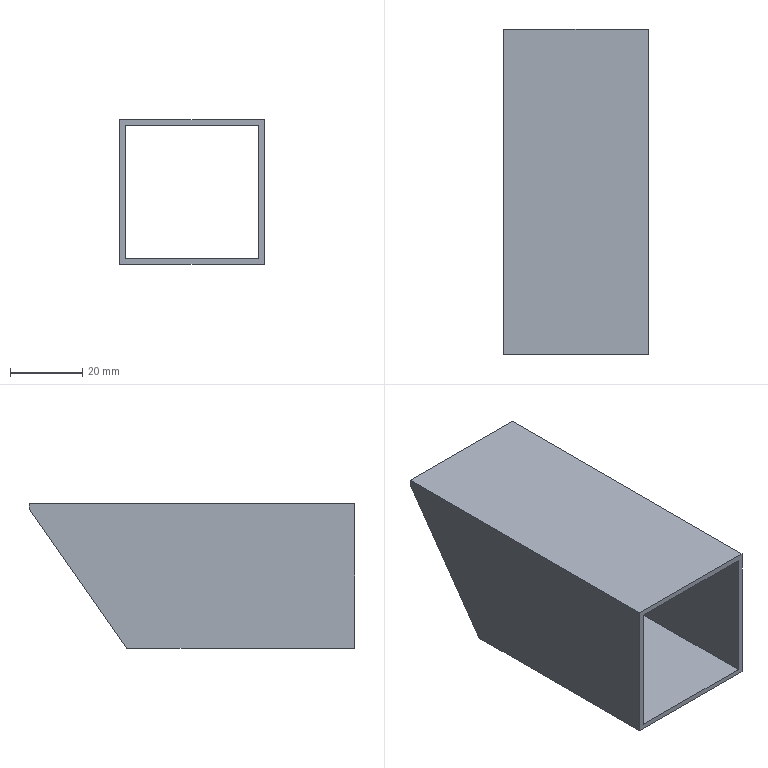Part | STEP file | 101 | 1 solid | 11 faces | box 40 x 90 x 40 mm | volume 17766 mm3 | plane 11
STEP:
#1=CARTESIAN_POINT('',(0.,0.,0.));
#2=DIRECTION('',(0.,0.,1.));
#3=DIRECTION('',(1.,0.,0.));
#4=AXIS2_PLACEMENT_3D('',#1,#2,#3);
#5=CARTESIAN_POINT('',(-20.,90.,18.5));
#6=VERTEX_POINT('',#5);
#7=CARTESIAN_POINT('',(-18.5,90.,18.5));
#8=VERTEX_POINT('',#7);
#9=CARTESIAN_POINT('',(0.,90.,18.5));
#10=DIRECTION('',(1.,0.,0.));
#11=VECTOR('',#10,1.);
#12=LINE('',#9,#11);
#13=CARTESIAN_POINT('',(0.,90.,0.));
#14=DIRECTION('',(0.,1.,0.));
#15=DIRECTION('',(0.,0.,1.));
#16=AXIS2_PLACEMENT_3D('',#13,#14,#15);
#17=PLANE('',#16);
#18=CARTESIAN_POINT('',(18.5,0.));
#19=DIRECTION('',(0.,1.));
#20=VECTOR('',#19,1.);
#21=LINE('',#18,#20);
#22=(GEOMETRIC_REPRESENTATION_CONTEXT(2)PARAMETRIC_REPRESENTATION_CONTEXT()REPRESENTATION_CONTEXT('',''));
#23=DEFINITIONAL_REPRESENTATION('',(#21),#22);
#24=PCURVE('',#17,#23);
#25=CARTESIAN_POINT('',(0.,51.699,-36.2));
#26=DIRECTION('',(0.,-0.8192,0.5736));
#27=DIRECTION('',(0.,-0.5736,-0.8192));
#28=AXIS2_PLACEMENT_3D('',#25,#26,#27);
#29=PLANE('',#28);
#30=CARTESIAN_POINT('',(-66.776,0.));
#31=DIRECTION('',(0.,1.));
#32=VECTOR('',#31,1.);
#33=LINE('',#30,#32);
#34=(GEOMETRIC_REPRESENTATION_CONTEXT(2)PARAMETRIC_REPRESENTATION_CONTEXT()REPRESENTATION_CONTEXT('',''));
#35=DEFINITIONAL_REPRESENTATION('',(#33),#34);
#36=PCURVE('',#29,#35);
#37=SURFACE_CURVE('',#12,(#24,#36),.PCURVE_S1.);
#38=EDGE_CURVE('',#6,#8,#37,.T.);
#39=ORIENTED_EDGE('',*,*,#38,.F.);
#40=CARTESIAN_POINT('',(-20.,90.,20.));
#41=VERTEX_POINT('',#40);
#42=CARTESIAN_POINT('',(-20.,90.,-20.));
#43=DIRECTION('',(0.,0.,1.));
#44=VECTOR('',#43,1.);
#45=LINE('',#42,#44);
#46=CARTESIAN_POINT('',(-20.,-20.));
#47=DIRECTION('',(1.,0.));
#48=VECTOR('',#47,1.);
#49=LINE('',#46,#48);
#50=(GEOMETRIC_REPRESENTATION_CONTEXT(2)PARAMETRIC_REPRESENTATION_CONTEXT()REPRESENTATION_CONTEXT('',''));
#51=DEFINITIONAL_REPRESENTATION('',(#49),#50);
#52=PCURVE('',#17,#51);
#53=CARTESIAN_POINT('',(-20.,90.,-20.));
#54=DIRECTION('',(1.,0.,0.));
#55=DIRECTION('',(0.,0.,-1.));
#56=AXIS2_PLACEMENT_3D('',#53,#54,#55);
#57=PLANE('',#56);
#58=CARTESIAN_POINT('',(0.,0.));
#59=DIRECTION('',(-1.,0.));
#60=VECTOR('',#59,1.);
#61=LINE('',#58,#60);
#62=(GEOMETRIC_REPRESENTATION_CONTEXT(2)PARAMETRIC_REPRESENTATION_CONTEXT()REPRESENTATION_CONTEXT('',''));
#63=DEFINITIONAL_REPRESENTATION('',(#61),#62);
#64=PCURVE('',#57,#63);
#65=SURFACE_CURVE('',#45,(#52,#64),.PCURVE_S1.);
#66=EDGE_CURVE('',#6,#41,#65,.T.);
#67=ORIENTED_EDGE('',*,*,#66,.T.);
#68=CARTESIAN_POINT('',(20.,90.,20.));
#69=VERTEX_POINT('',#68);
#70=CARTESIAN_POINT('',(-20.,90.,20.));
#71=DIRECTION('',(1.,0.,0.));
#72=VECTOR('',#71,1.);
#73=LINE('',#70,#72);
#74=CARTESIAN_POINT('',(20.,-20.));
#75=DIRECTION('',(0.,1.));
#76=VECTOR('',#75,1.);
#77=LINE('',#74,#76);
#78=(GEOMETRIC_REPRESENTATION_CONTEXT(2)PARAMETRIC_REPRESENTATION_CONTEXT()REPRESENTATION_CONTEXT('',''));
#79=DEFINITIONAL_REPRESENTATION('',(#77),#78);
#80=PCURVE('',#17,#79);
#81=CARTESIAN_POINT('',(-20.,90.,20.));
#82=DIRECTION('',(0.,0.,-1.));
#83=DIRECTION('',(-1.,0.,0.));
#84=AXIS2_PLACEMENT_3D('',#81,#82,#83);
#85=PLANE('',#84);
#86=CARTESIAN_POINT('',(0.,0.));
#87=DIRECTION('',(-1.,0.));
#88=VECTOR('',#87,1.);
#89=LINE('',#86,#88);
#90=(GEOMETRIC_REPRESENTATION_CONTEXT(2)PARAMETRIC_REPRESENTATION_CONTEXT()REPRESENTATION_CONTEXT('',''));
#91=DEFINITIONAL_REPRESENTATION('',(#89),#90);
#92=PCURVE('',#85,#91);
#93=SURFACE_CURVE('',#73,(#80,#92),.PCURVE_S1.);
#94=EDGE_CURVE('',#41,#69,#93,.T.);
#95=ORIENTED_EDGE('',*,*,#94,.T.);
#96=CARTESIAN_POINT('',(20.,90.,18.5));
#97=VERTEX_POINT('',#96);
#98=CARTESIAN_POINT('',(20.,90.,-20.));
#99=DIRECTION('',(0.,0.,-1.));
#100=VECTOR('',#99,1.);
#101=LINE('',#98,#100);
#102=CARTESIAN_POINT('',(-20.,20.));
#103=DIRECTION('',(-1.,0.));
#104=VECTOR('',#103,1.);
#105=LINE('',#102,#104);
#106=(GEOMETRIC_REPRESENTATION_CONTEXT(2)PARAMETRIC_REPRESENTATION_CONTEXT()REPRESENTATION_CONTEXT('',''));
#107=DEFINITIONAL_REPRESENTATION('',(#105),#106);
#108=PCURVE('',#17,#107);
#109=CARTESIAN_POINT('',(20.,90.,-20.));
#110=DIRECTION('',(-1.,0.,0.));
#111=DIRECTION('',(0.,0.,1.));
#112=AXIS2_PLACEMENT_3D('',#109,#110,#111);
#113=PLANE('',#112);
#114=CARTESIAN_POINT('',(0.,0.));
#115=DIRECTION('',(-1.,0.));
#116=VECTOR('',#115,1.);
#117=LINE('',#114,#116);
#118=(GEOMETRIC_REPRESENTATION_CONTEXT(2)PARAMETRIC_REPRESENTATION_CONTEXT()REPRESENTATION_CONTEXT('',''));
#119=DEFINITIONAL_REPRESENTATION('',(#117),#118);
#120=PCURVE('',#113,#119);
#121=SURFACE_CURVE('',#101,(#108,#120),.PCURVE_S1.);
#122=EDGE_CURVE('',#69,#97,#121,.T.);
#123=ORIENTED_EDGE('',*,*,#122,.T.);
#124=CARTESIAN_POINT('',(18.5,90.,18.5));
#125=VERTEX_POINT('',#124);
#126=CARTESIAN_POINT('',(0.,90.,18.5));
#127=DIRECTION('',(1.,0.,0.));
#128=VECTOR('',#127,1.);
#129=LINE('',#126,#128);
#130=CARTESIAN_POINT('',(18.5,0.));
#131=DIRECTION('',(0.,1.));
#132=VECTOR('',#131,1.);
#133=LINE('',#130,#132);
#134=(GEOMETRIC_REPRESENTATION_CONTEXT(2)PARAMETRIC_REPRESENTATION_CONTEXT()REPRESENTATION_CONTEXT('',''));
#135=DEFINITIONAL_REPRESENTATION('',(#133),#134);
#136=PCURVE('',#17,#135);
#137=CARTESIAN_POINT('',(-66.776,0.));
#138=DIRECTION('',(0.,1.));
#139=VECTOR('',#138,1.);
#140=LINE('',#137,#139);
#141=(GEOMETRIC_REPRESENTATION_CONTEXT(2)PARAMETRIC_REPRESENTATION_CONTEXT()REPRESENTATION_CONTEXT('',''));
#142=DEFINITIONAL_REPRESENTATION('',(#140),#141);
#143=PCURVE('',#29,#142);
#144=SURFACE_CURVE('',#129,(#136,#143),.PCURVE_S1.);
#145=EDGE_CURVE('',#125,#97,#144,.T.);
#146=ORIENTED_EDGE('',*,*,#145,.F.);
#147=CARTESIAN_POINT('',(-18.5,90.,18.5));
#148=DIRECTION('',(1.,0.,0.));
#149=VECTOR('',#148,1.);
#150=LINE('',#147,#149);
#151=CARTESIAN_POINT('',(18.5,-18.5));
#152=DIRECTION('',(0.,1.));
#153=VECTOR('',#152,1.);
#154=LINE('',#151,#153);
#155=(GEOMETRIC_REPRESENTATION_CONTEXT(2)PARAMETRIC_REPRESENTATION_CONTEXT()REPRESENTATION_CONTEXT('',''));
#156=DEFINITIONAL_REPRESENTATION('',(#154),#155);
#157=PCURVE('',#17,#156);
#158=CARTESIAN_POINT('',(-18.5,90.,18.5));
#159=DIRECTION('',(0.,0.,-1.));
#160=DIRECTION('',(-1.,0.,0.));
#161=AXIS2_PLACEMENT_3D('',#158,#159,#160);
#162=PLANE('',#161);
#163=CARTESIAN_POINT('',(0.,0.));
#164=DIRECTION('',(-1.,0.));
#165=VECTOR('',#164,1.);
#166=LINE('',#163,#165);
#167=(GEOMETRIC_REPRESENTATION_CONTEXT(2)PARAMETRIC_REPRESENTATION_CONTEXT()REPRESENTATION_CONTEXT('',''));
#168=DEFINITIONAL_REPRESENTATION('',(#166),#167);
#169=PCURVE('',#162,#168);
#170=SURFACE_CURVE('',#150,(#157,#169),.PCURVE_S1.);
#171=EDGE_CURVE('',#8,#125,#170,.T.);
#172=ORIENTED_EDGE('',*,*,#171,.F.);
#173=EDGE_LOOP('',(#39,#67,#95,#123,#146,#172));
#174=FACE_BOUND('',#173,.T.);
#175=ADVANCED_FACE('',(#174),#17,.T.);
#176=CARTESIAN_POINT('',(20.,0.,20.));
#177=VERTEX_POINT('',#176);
#178=CARTESIAN_POINT('',(20.,0.,-20.));
#179=VERTEX_POINT('',#178);
#180=CARTESIAN_POINT('',(20.,0.,-20.));
#181=DIRECTION('',(0.,0.,-1.));
#182=VECTOR('',#181,1.);
#183=LINE('',#180,#182);
#184=CARTESIAN_POINT('',(0.,0.,0.));
#185=DIRECTION('',(0.,1.,0.));
#186=DIRECTION('',(0.,0.,1.));
#187=AXIS2_PLACEMENT_3D('',#184,#185,#186);
#188=PLANE('',#187);
#189=CARTESIAN_POINT('',(-20.,20.));
#190=DIRECTION('',(-1.,0.));
#191=VECTOR('',#190,1.);
#192=LINE('',#189,#191);
#193=(GEOMETRIC_REPRESENTATION_CONTEXT(2)PARAMETRIC_REPRESENTATION_CONTEXT()REPRESENTATION_CONTEXT('',''));
#194=DEFINITIONAL_REPRESENTATION('',(#192),#193);
#195=PCURVE('',#188,#194);
#196=CARTESIAN_POINT('',(0.,-90.));
#197=DIRECTION('',(-1.,0.));
#198=VECTOR('',#197,1.);
#199=LINE('',#196,#198);
#200=(GEOMETRIC_REPRESENTATION_CONTEXT(2)PARAMETRIC_REPRESENTATION_CONTEXT()REPRESENTATION_CONTEXT('',''));
#201=DEFINITIONAL_REPRESENTATION('',(#199),#200);
#202=PCURVE('',#113,#201);
#203=SURFACE_CURVE('',#183,(#195,#202),.PCURVE_S1.);
#204=EDGE_CURVE('',#177,#179,#203,.T.);
#205=ORIENTED_EDGE('',*,*,#204,.F.);
#206=CARTESIAN_POINT('',(-20.,0.,20.));
#207=VERTEX_POINT('',#206);
#208=CARTESIAN_POINT('',(-20.,0.,20.));
#209=DIRECTION('',(1.,0.,0.));
#210=VECTOR('',#209,1.);
#211=LINE('',#208,#210);
#212=CARTESIAN_POINT('',(20.,-20.));
#213=DIRECTION('',(0.,1.));
#214=VECTOR('',#213,1.);
#215=LINE('',#212,#214);
#216=(GEOMETRIC_REPRESENTATION_CONTEXT(2)PARAMETRIC_REPRESENTATION_CONTEXT()REPRESENTATION_CONTEXT('',''));
#217=DEFINITIONAL_REPRESENTATION('',(#215),#216);
#218=PCURVE('',#188,#217);
#219=CARTESIAN_POINT('',(0.,-90.));
#220=DIRECTION('',(-1.,0.));
#221=VECTOR('',#220,1.);
#222=LINE('',#219,#221);
#223=(GEOMETRIC_REPRESENTATION_CONTEXT(2)PARAMETRIC_REPRESENTATION_CONTEXT()REPRESENTATION_CONTEXT('',''));
#224=DEFINITIONAL_REPRESENTATION('',(#222),#223);
#225=PCURVE('',#85,#224);
#226=SURFACE_CURVE('',#211,(#218,#225),.PCURVE_S1.);
#227=EDGE_CURVE('',#207,#177,#226,.T.);
#228=ORIENTED_EDGE('',*,*,#227,.F.);
#229=CARTESIAN_POINT('',(-20.,0.,-20.));
#230=VERTEX_POINT('',#229);
#231=CARTESIAN_POINT('',(-20.,0.,-20.));
#232=DIRECTION('',(0.,0.,1.));
#233=VECTOR('',#232,1.);
#234=LINE('',#231,#233);
#235=CARTESIAN_POINT('',(-20.,-20.));
#236=DIRECTION('',(1.,0.));
#237=VECTOR('',#236,1.);
#238=LINE('',#235,#237);
#239=(GEOMETRIC_REPRESENTATION_CONTEXT(2)PARAMETRIC_REPRESENTATION_CONTEXT()REPRESENTATION_CONTEXT('',''));
#240=DEFINITIONAL_REPRESENTATION('',(#238),#239);
#241=PCURVE('',#188,#240);
#242=CARTESIAN_POINT('',(0.,-90.));
#243=DIRECTION('',(-1.,0.));
#244=VECTOR('',#243,1.);
#245=LINE('',#242,#244);
#246=(GEOMETRIC_REPRESENTATION_CONTEXT(2)PARAMETRIC_REPRESENTATION_CONTEXT()REPRESENTATION_CONTEXT('',''));
#247=DEFINITIONAL_REPRESENTATION('',(#245),#246);
#248=PCURVE('',#57,#247);
#249=SURFACE_CURVE('',#234,(#241,#248),.PCURVE_S1.);
#250=EDGE_CURVE('',#230,#207,#249,.T.);
#251=ORIENTED_EDGE('',*,*,#250,.F.);
#252=CARTESIAN_POINT('',(-20.,0.,-20.));
#253=DIRECTION('',(-1.,0.,0.));
#254=VECTOR('',#253,1.);
#255=LINE('',#252,#254);
#256=CARTESIAN_POINT('',(-20.,-20.));
#257=DIRECTION('',(0.,-1.));
#258=VECTOR('',#257,1.);
#259=LINE('',#256,#258);
#260=(GEOMETRIC_REPRESENTATION_CONTEXT(2)PARAMETRIC_REPRESENTATION_CONTEXT()REPRESENTATION_CONTEXT('',''));
#261=DEFINITIONAL_REPRESENTATION('',(#259),#260);
#262=PCURVE('',#188,#261);
#263=CARTESIAN_POINT('',(-20.,90.,-20.));
#264=DIRECTION('',(0.,0.,1.));
#265=DIRECTION('',(1.,0.,0.));
#266=AXIS2_PLACEMENT_3D('',#263,#264,#265);
#267=PLANE('',#266);
#268=CARTESIAN_POINT('',(0.,-90.));
#269=DIRECTION('',(-1.,0.));
#270=VECTOR('',#269,1.);
#271=LINE('',#268,#270);
#272=(GEOMETRIC_REPRESENTATION_CONTEXT(2)PARAMETRIC_REPRESENTATION_CONTEXT()REPRESENTATION_CONTEXT('',''));
#273=DEFINITIONAL_REPRESENTATION('',(#271),#272);
#274=PCURVE('',#267,#273);
#275=SURFACE_CURVE('',#255,(#262,#274),.PCURVE_S1.);
#276=EDGE_CURVE('',#179,#230,#275,.T.);
#277=ORIENTED_EDGE('',*,*,#276,.F.);
#278=EDGE_LOOP('',(#205,#228,#251,#277));
#279=FACE_BOUND('',#278,.T.);
#280=CARTESIAN_POINT('',(18.5,0.,18.5));
#281=VERTEX_POINT('',#280);
#282=CARTESIAN_POINT('',(18.5,0.,-18.5));
#283=VERTEX_POINT('',#282);
#284=CARTESIAN_POINT('',(18.5,0.,-18.5));
#285=DIRECTION('',(0.,0.,-1.));
#286=VECTOR('',#285,1.);
#287=LINE('',#284,#286);
#288=CARTESIAN_POINT('',(-18.5,18.5));
#289=DIRECTION('',(-1.,0.));
#290=VECTOR('',#289,1.);
#291=LINE('',#288,#290);
#292=(GEOMETRIC_REPRESENTATION_CONTEXT(2)PARAMETRIC_REPRESENTATION_CONTEXT()REPRESENTATION_CONTEXT('',''));
#293=DEFINITIONAL_REPRESENTATION('',(#291),#292);
#294=PCURVE('',#188,#293);
#295=CARTESIAN_POINT('',(18.5,90.,-18.5));
#296=DIRECTION('',(-1.,0.,0.));
#297=DIRECTION('',(0.,0.,1.));
#298=AXIS2_PLACEMENT_3D('',#295,#296,#297);
#299=PLANE('',#298);
#300=CARTESIAN_POINT('',(0.,-90.));
#301=DIRECTION('',(-1.,0.));
#302=VECTOR('',#301,1.);
#303=LINE('',#300,#302);
#304=(GEOMETRIC_REPRESENTATION_CONTEXT(2)PARAMETRIC_REPRESENTATION_CONTEXT()REPRESENTATION_CONTEXT('',''));
#305=DEFINITIONAL_REPRESENTATION('',(#303),#304);
#306=PCURVE('',#299,#305);
#307=SURFACE_CURVE('',#287,(#294,#306),.PCURVE_S1.);
#308=EDGE_CURVE('',#281,#283,#307,.T.);
#309=ORIENTED_EDGE('',*,*,#308,.T.);
#310=CARTESIAN_POINT('',(-18.5,0.,-18.5));
#311=VERTEX_POINT('',#310);
#312=CARTESIAN_POINT('',(-18.5,0.,-18.5));
#313=DIRECTION('',(-1.,0.,0.));
#314=VECTOR('',#313,1.);
#315=LINE('',#312,#314);
#316=CARTESIAN_POINT('',(-18.5,-18.5));
#317=DIRECTION('',(0.,-1.));
#318=VECTOR('',#317,1.);
#319=LINE('',#316,#318);
#320=(GEOMETRIC_REPRESENTATION_CONTEXT(2)PARAMETRIC_REPRESENTATION_CONTEXT()REPRESENTATION_CONTEXT('',''));
#321=DEFINITIONAL_REPRESENTATION('',(#319),#320);
#322=PCURVE('',#188,#321);
#323=CARTESIAN_POINT('',(-18.5,90.,-18.5));
#324=DIRECTION('',(0.,0.,1.));
#325=DIRECTION('',(1.,0.,0.));
#326=AXIS2_PLACEMENT_3D('',#323,#324,#325);
#327=PLANE('',#326);
#328=CARTESIAN_POINT('',(0.,-90.));
#329=DIRECTION('',(-1.,0.));
#330=VECTOR('',#329,1.);
#331=LINE('',#328,#330);
#332=(GEOMETRIC_REPRESENTATION_CONTEXT(2)PARAMETRIC_REPRESENTATION_CONTEXT()REPRESENTATION_CONTEXT('',''));
#333=DEFINITIONAL_REPRESENTATION('',(#331),#332);
#334=PCURVE('',#327,#333);
#335=SURFACE_CURVE('',#315,(#322,#334),.PCURVE_S1.);
#336=EDGE_CURVE('',#283,#311,#335,.T.);
#337=ORIENTED_EDGE('',*,*,#336,.T.);
#338=CARTESIAN_POINT('',(-18.5,0.,18.5));
#339=VERTEX_POINT('',#338);
#340=CARTESIAN_POINT('',(-18.5,0.,-18.5));
#341=DIRECTION('',(0.,0.,1.));
#342=VECTOR('',#341,1.);
#343=LINE('',#340,#342);
#344=CARTESIAN_POINT('',(-18.5,-18.5));
#345=DIRECTION('',(1.,0.));
#346=VECTOR('',#345,1.);
#347=LINE('',#344,#346);
#348=(GEOMETRIC_REPRESENTATION_CONTEXT(2)PARAMETRIC_REPRESENTATION_CONTEXT()REPRESENTATION_CONTEXT('',''));
#349=DEFINITIONAL_REPRESENTATION('',(#347),#348);
#350=PCURVE('',#188,#349);
#351=CARTESIAN_POINT('',(-18.5,90.,-18.5));
#352=DIRECTION('',(1.,0.,0.));
#353=DIRECTION('',(0.,0.,-1.));
#354=AXIS2_PLACEMENT_3D('',#351,#352,#353);
#355=PLANE('',#354);
#356=CARTESIAN_POINT('',(0.,-90.));
#357=DIRECTION('',(-1.,0.));
#358=VECTOR('',#357,1.);
#359=LINE('',#356,#358);
#360=(GEOMETRIC_REPRESENTATION_CONTEXT(2)PARAMETRIC_REPRESENTATION_CONTEXT()REPRESENTATION_CONTEXT('',''));
#361=DEFINITIONAL_REPRESENTATION('',(#359),#360);
#362=PCURVE('',#355,#361);
#363=SURFACE_CURVE('',#343,(#350,#362),.PCURVE_S1.);
#364=EDGE_CURVE('',#311,#339,#363,.T.);
#365=ORIENTED_EDGE('',*,*,#364,.T.);
#366=CARTESIAN_POINT('',(-18.5,0.,18.5));
#367=DIRECTION('',(1.,0.,0.));
#368=VECTOR('',#367,1.);
#369=LINE('',#366,#368);
#370=CARTESIAN_POINT('',(18.5,-18.5));
#371=DIRECTION('',(0.,1.));
#372=VECTOR('',#371,1.);
#373=LINE('',#370,#372);
#374=(GEOMETRIC_REPRESENTATION_CONTEXT(2)PARAMETRIC_REPRESENTATION_CONTEXT()REPRESENTATION_CONTEXT('',''));
#375=DEFINITIONAL_REPRESENTATION('',(#373),#374);
#376=PCURVE('',#188,#375);
#377=CARTESIAN_POINT('',(0.,-90.));
#378=DIRECTION('',(-1.,0.));
#379=VECTOR('',#378,1.);
#380=LINE('',#377,#379);
#381=(GEOMETRIC_REPRESENTATION_CONTEXT(2)PARAMETRIC_REPRESENTATION_CONTEXT()REPRESENTATION_CONTEXT('',''));
#382=DEFINITIONAL_REPRESENTATION('',(#380),#381);
#383=PCURVE('',#162,#382);
#384=SURFACE_CURVE('',#369,(#376,#383),.PCURVE_S1.);
#385=EDGE_CURVE('',#339,#281,#384,.T.);
#386=ORIENTED_EDGE('',*,*,#385,.T.);
#387=EDGE_LOOP('',(#309,#337,#365,#386));
#388=FACE_BOUND('',#387,.T.);
#389=ADVANCED_FACE('',(#279,#388),#188,.F.);
#390=CARTESIAN_POINT('',(20.,63.042,-20.));
#391=VERTEX_POINT('',#390);
#392=CARTESIAN_POINT('',(20.,90.,-20.));
#393=DIRECTION('',(0.,-1.,0.));
#394=VECTOR('',#393,1.);
#395=LINE('',#392,#394);
#396=CARTESIAN_POINT('',(0.,0.));
#397=DIRECTION('',(0.,-1.));
#398=VECTOR('',#397,1.);
#399=LINE('',#396,#398);
#400=(GEOMETRIC_REPRESENTATION_CONTEXT(2)PARAMETRIC_REPRESENTATION_CONTEXT()REPRESENTATION_CONTEXT('',''));
#401=DEFINITIONAL_REPRESENTATION('',(#399),#400);
#402=PCURVE('',#113,#401);
#403=CARTESIAN_POINT('',(40.,0.));
#404=DIRECTION('',(0.,-1.));
#405=VECTOR('',#404,1.);
#406=LINE('',#403,#405);
#407=(GEOMETRIC_REPRESENTATION_CONTEXT(2)PARAMETRIC_REPRESENTATION_CONTEXT()REPRESENTATION_CONTEXT('',''));
#408=DEFINITIONAL_REPRESENTATION('',(#406),#407);
#409=PCURVE('',#267,#408);
#410=SURFACE_CURVE('',#395,(#402,#409),.PCURVE_S1.);
#411=EDGE_CURVE('',#391,#179,#410,.T.);
#412=ORIENTED_EDGE('',*,*,#411,.F.);
#413=CARTESIAN_POINT('',(20.,71.911,-7.334));
#414=DIRECTION('',(0.,0.5736,0.8192));
#415=VECTOR('',#414,1.);
#416=LINE('',#413,#415);
#417=CARTESIAN_POINT('',(12.666,-18.089));
#418=DIRECTION('',(0.8192,0.5736));
#419=VECTOR('',#418,1.);
#420=LINE('',#417,#419);
#421=(GEOMETRIC_REPRESENTATION_CONTEXT(2)PARAMETRIC_REPRESENTATION_CONTEXT()REPRESENTATION_CONTEXT('',''));
#422=DEFINITIONAL_REPRESENTATION('',(#420),#421);
#423=PCURVE('',#113,#422);
#424=CARTESIAN_POINT('',(-35.239,20.));
#425=DIRECTION('',(-1.,0.));
#426=VECTOR('',#425,1.);
#427=LINE('',#424,#426);
#428=(GEOMETRIC_REPRESENTATION_CONTEXT(2)PARAMETRIC_REPRESENTATION_CONTEXT()REPRESENTATION_CONTEXT('',''));
#429=DEFINITIONAL_REPRESENTATION('',(#427),#428);
#430=PCURVE('',#29,#429);
#431=SURFACE_CURVE('',#416,(#423,#430),.PCURVE_S1.);
#432=EDGE_CURVE('',#391,#97,#431,.T.);
#433=ORIENTED_EDGE('',*,*,#432,.T.);
#434=ORIENTED_EDGE('',*,*,#122,.F.);
#435=CARTESIAN_POINT('',(20.,90.,20.));
#436=DIRECTION('',(0.,-1.,0.));
#437=VECTOR('',#436,1.);
#438=LINE('',#435,#437);
#439=CARTESIAN_POINT('',(40.,0.));
#440=DIRECTION('',(0.,-1.));
#441=VECTOR('',#440,1.);
#442=LINE('',#439,#441);
#443=(GEOMETRIC_REPRESENTATION_CONTEXT(2)PARAMETRIC_REPRESENTATION_CONTEXT()REPRESENTATION_CONTEXT('',''));
#444=DEFINITIONAL_REPRESENTATION('',(#442),#443);
#445=PCURVE('',#113,#444);
#446=CARTESIAN_POINT('',(-40.,0.));
#447=DIRECTION('',(0.,-1.));
#448=VECTOR('',#447,1.);
#449=LINE('',#446,#448);
#450=(GEOMETRIC_REPRESENTATION_CONTEXT(2)PARAMETRIC_REPRESENTATION_CONTEXT()REPRESENTATION_CONTEXT('',''));
#451=DEFINITIONAL_REPRESENTATION('',(#449),#450);
#452=PCURVE('',#85,#451);
#453=SURFACE_CURVE('',#438,(#445,#452),.PCURVE_S1.);
#454=EDGE_CURVE('',#69,#177,#453,.T.);
#455=ORIENTED_EDGE('',*,*,#454,.T.);
#456=ORIENTED_EDGE('',*,*,#204,.T.);
#457=EDGE_LOOP('',(#412,#433,#434,#455,#456));
#458=FACE_BOUND('',#457,.T.);
#459=ADVANCED_FACE('',(#458),#113,.F.);
#460=CARTESIAN_POINT('',(-20.,63.042,-20.));
#461=VERTEX_POINT('',#460);
#462=CARTESIAN_POINT('',(-20.,90.,-20.));
#463=DIRECTION('',(0.,-1.,0.));
#464=VECTOR('',#463,1.);
#465=LINE('',#462,#464);
#466=CARTESIAN_POINT('',(0.,0.));
#467=DIRECTION('',(0.,-1.));
#468=VECTOR('',#467,1.);
#469=LINE('',#466,#468);
#470=(GEOMETRIC_REPRESENTATION_CONTEXT(2)PARAMETRIC_REPRESENTATION_CONTEXT()REPRESENTATION_CONTEXT('',''));
#471=DEFINITIONAL_REPRESENTATION('',(#469),#470);
#472=PCURVE('',#267,#471);
#473=CARTESIAN_POINT('',(0.,0.));
#474=DIRECTION('',(0.,-1.));
#475=VECTOR('',#474,1.);
#476=LINE('',#473,#475);
#477=(GEOMETRIC_REPRESENTATION_CONTEXT(2)PARAMETRIC_REPRESENTATION_CONTEXT()REPRESENTATION_CONTEXT('',''));
#478=DEFINITIONAL_REPRESENTATION('',(#476),#477);
#479=PCURVE('',#57,#478);
#480=SURFACE_CURVE('',#465,(#472,#479),.PCURVE_S1.);
#481=EDGE_CURVE('',#461,#230,#480,.T.);
#482=ORIENTED_EDGE('',*,*,#481,.F.);
#483=CARTESIAN_POINT('',(-20.,63.042,-20.));
#484=DIRECTION('',(1.,0.,0.));
#485=VECTOR('',#484,1.);
#486=LINE('',#483,#485);
#487=CARTESIAN_POINT('',(0.,-26.958));
#488=DIRECTION('',(1.,0.));
#489=VECTOR('',#488,1.);
#490=LINE('',#487,#489);
#491=(GEOMETRIC_REPRESENTATION_CONTEXT(2)PARAMETRIC_REPRESENTATION_CONTEXT()REPRESENTATION_CONTEXT('',''));
#492=DEFINITIONAL_REPRESENTATION('',(#490),#491);
#493=PCURVE('',#267,#492);
#494=CARTESIAN_POINT('',(-19.776,-20.));
#495=DIRECTION('',(0.,1.));
#496=VECTOR('',#495,1.);
#497=LINE('',#494,#496);
#498=(GEOMETRIC_REPRESENTATION_CONTEXT(2)PARAMETRIC_REPRESENTATION_CONTEXT()REPRESENTATION_CONTEXT('',''));
#499=DEFINITIONAL_REPRESENTATION('',(#497),#498);
#500=PCURVE('',#29,#499);
#501=SURFACE_CURVE('',#486,(#493,#500),.PCURVE_S1.);
#502=EDGE_CURVE('',#461,#391,#501,.T.);
#503=ORIENTED_EDGE('',*,*,#502,.T.);
#504=ORIENTED_EDGE('',*,*,#411,.T.);
#505=ORIENTED_EDGE('',*,*,#276,.T.);
#506=EDGE_LOOP('',(#482,#503,#504,#505));
#507=FACE_BOUND('',#506,.T.);
#508=ADVANCED_FACE('',(#507),#267,.F.);
#509=ORIENTED_EDGE('',*,*,#66,.F.);
#510=CARTESIAN_POINT('',(-20.,71.911,-7.334));
#511=DIRECTION('',(0.,-0.5736,-0.8192));
#512=VECTOR('',#511,1.);
#513=LINE('',#510,#512);
#514=CARTESIAN_POINT('',(-12.666,-18.089));
#515=DIRECTION('',(0.8192,-0.5736));
#516=VECTOR('',#515,1.);
#517=LINE('',#514,#516);
#518=(GEOMETRIC_REPRESENTATION_CONTEXT(2)PARAMETRIC_REPRESENTATION_CONTEXT()REPRESENTATION_CONTEXT('',''));
#519=DEFINITIONAL_REPRESENTATION('',(#517),#518);
#520=PCURVE('',#57,#519);
#521=CARTESIAN_POINT('',(-35.239,-20.));
#522=DIRECTION('',(1.,0.));
#523=VECTOR('',#522,1.);
#524=LINE('',#521,#523);
#525=(GEOMETRIC_REPRESENTATION_CONTEXT(2)PARAMETRIC_REPRESENTATION_CONTEXT()REPRESENTATION_CONTEXT('',''));
#526=DEFINITIONAL_REPRESENTATION('',(#524),#525);
#527=PCURVE('',#29,#526);
#528=SURFACE_CURVE('',#513,(#520,#527),.PCURVE_S1.);
#529=EDGE_CURVE('',#6,#461,#528,.T.);
#530=ORIENTED_EDGE('',*,*,#529,.T.);
#531=ORIENTED_EDGE('',*,*,#481,.T.);
#532=ORIENTED_EDGE('',*,*,#250,.T.);
#533=CARTESIAN_POINT('',(-20.,90.,20.));
#534=DIRECTION('',(0.,-1.,0.));
#535=VECTOR('',#534,1.);
#536=LINE('',#533,#535);
#537=CARTESIAN_POINT('',(-40.,0.));
#538=DIRECTION('',(0.,-1.));
#539=VECTOR('',#538,1.);
#540=LINE('',#537,#539);
#541=(GEOMETRIC_REPRESENTATION_CONTEXT(2)PARAMETRIC_REPRESENTATION_CONTEXT()REPRESENTATION_CONTEXT('',''));
#542=DEFINITIONAL_REPRESENTATION('',(#540),#541);
#543=PCURVE('',#57,#542);
#544=CARTESIAN_POINT('',(0.,0.));
#545=DIRECTION('',(0.,-1.));
#546=VECTOR('',#545,1.);
#547=LINE('',#544,#546);
#548=(GEOMETRIC_REPRESENTATION_CONTEXT(2)PARAMETRIC_REPRESENTATION_CONTEXT()REPRESENTATION_CONTEXT('',''));
#549=DEFINITIONAL_REPRESENTATION('',(#547),#548);
#550=PCURVE('',#85,#549);
#551=SURFACE_CURVE('',#536,(#543,#550),.PCURVE_S1.);
#552=EDGE_CURVE('',#41,#207,#551,.T.);
#553=ORIENTED_EDGE('',*,*,#552,.F.);
#554=EDGE_LOOP('',(#509,#530,#531,#532,#553));
#555=FACE_BOUND('',#554,.T.);
#556=ADVANCED_FACE('',(#555),#57,.F.);
#557=ORIENTED_EDGE('',*,*,#227,.T.);
#558=ORIENTED_EDGE('',*,*,#454,.F.);
#559=ORIENTED_EDGE('',*,*,#94,.F.);
#560=ORIENTED_EDGE('',*,*,#552,.T.);
#561=EDGE_LOOP('',(#557,#558,#559,#560));
#562=FACE_BOUND('',#561,.T.);
#563=ADVANCED_FACE('',(#562),#85,.F.);
#564=CARTESIAN_POINT('',(18.5,64.092,-18.5));
#565=VERTEX_POINT('',#564);
#566=CARTESIAN_POINT('',(18.5,72.616,-6.327));
#567=DIRECTION('',(0.,0.5736,0.8192));
#568=VECTOR('',#567,1.);
#569=LINE('',#566,#568);
#570=CARTESIAN_POINT('',(12.173,-17.384));
#571=DIRECTION('',(0.8192,0.5736));
#572=VECTOR('',#571,1.);
#573=LINE('',#570,#572);
#574=(GEOMETRIC_REPRESENTATION_CONTEXT(2)PARAMETRIC_REPRESENTATION_CONTEXT()REPRESENTATION_CONTEXT('',''));
#575=DEFINITIONAL_REPRESENTATION('',(#573),#574);
#576=PCURVE('',#299,#575);
#577=CARTESIAN_POINT('',(-36.468,18.5));
#578=DIRECTION('',(-1.,0.));
#579=VECTOR('',#578,1.);
#580=LINE('',#577,#579);
#581=(GEOMETRIC_REPRESENTATION_CONTEXT(2)PARAMETRIC_REPRESENTATION_CONTEXT()REPRESENTATION_CONTEXT('',''));
#582=DEFINITIONAL_REPRESENTATION('',(#580),#581);
#583=PCURVE('',#29,#582);
#584=SURFACE_CURVE('',#569,(#576,#583),.PCURVE_S1.);
#585=EDGE_CURVE('',#565,#125,#584,.T.);
#586=ORIENTED_EDGE('',*,*,#585,.F.);
#587=CARTESIAN_POINT('',(18.5,90.,-18.5));
#588=DIRECTION('',(0.,-1.,0.));
#589=VECTOR('',#588,1.);
#590=LINE('',#587,#589);
#591=CARTESIAN_POINT('',(0.,0.));
#592=DIRECTION('',(0.,-1.));
#593=VECTOR('',#592,1.);
#594=LINE('',#591,#593);
#595=(GEOMETRIC_REPRESENTATION_CONTEXT(2)PARAMETRIC_REPRESENTATION_CONTEXT()REPRESENTATION_CONTEXT('',''));
#596=DEFINITIONAL_REPRESENTATION('',(#594),#595);
#597=PCURVE('',#299,#596);
#598=CARTESIAN_POINT('',(37.,0.));
#599=DIRECTION('',(0.,-1.));
#600=VECTOR('',#599,1.);
#601=LINE('',#598,#600);
#602=(GEOMETRIC_REPRESENTATION_CONTEXT(2)PARAMETRIC_REPRESENTATION_CONTEXT()REPRESENTATION_CONTEXT('',''));
#603=DEFINITIONAL_REPRESENTATION('',(#601),#602);
#604=PCURVE('',#327,#603);
#605=SURFACE_CURVE('',#590,(#597,#604),.PCURVE_S1.);
#606=EDGE_CURVE('',#565,#283,#605,.T.);
#607=ORIENTED_EDGE('',*,*,#606,.T.);
#608=ORIENTED_EDGE('',*,*,#308,.F.);
#609=CARTESIAN_POINT('',(18.5,90.,18.5));
#610=DIRECTION('',(0.,-1.,0.));
#611=VECTOR('',#610,1.);
#612=LINE('',#609,#611);
#613=CARTESIAN_POINT('',(37.,0.));
#614=DIRECTION('',(0.,-1.));
#615=VECTOR('',#614,1.);
#616=LINE('',#613,#615);
#617=(GEOMETRIC_REPRESENTATION_CONTEXT(2)PARAMETRIC_REPRESENTATION_CONTEXT()REPRESENTATION_CONTEXT('',''));
#618=DEFINITIONAL_REPRESENTATION('',(#616),#617);
#619=PCURVE('',#299,#618);
#620=CARTESIAN_POINT('',(-37.,0.));
#621=DIRECTION('',(0.,-1.));
#622=VECTOR('',#621,1.);
#623=LINE('',#620,#622);
#624=(GEOMETRIC_REPRESENTATION_CONTEXT(2)PARAMETRIC_REPRESENTATION_CONTEXT()REPRESENTATION_CONTEXT('',''));
#625=DEFINITIONAL_REPRESENTATION('',(#623),#624);
#626=PCURVE('',#162,#625);
#627=SURFACE_CURVE('',#612,(#619,#626),.PCURVE_S1.);
#628=EDGE_CURVE('',#125,#281,#627,.T.);
#629=ORIENTED_EDGE('',*,*,#628,.F.);
#630=EDGE_LOOP('',(#586,#607,#608,#629));
#631=FACE_BOUND('',#630,.T.);
#632=ADVANCED_FACE('',(#631),#299,.T.);
#633=CARTESIAN_POINT('',(-18.5,64.092,-18.5));
#634=VERTEX_POINT('',#633);
#635=CARTESIAN_POINT('',(-18.5,64.092,-18.5));
#636=DIRECTION('',(1.,0.,0.));
#637=VECTOR('',#636,1.);
#638=LINE('',#635,#637);
#639=CARTESIAN_POINT('',(0.,-25.908));
#640=DIRECTION('',(1.,0.));
#641=VECTOR('',#640,1.);
#642=LINE('',#639,#641);
#643=(GEOMETRIC_REPRESENTATION_CONTEXT(2)PARAMETRIC_REPRESENTATION_CONTEXT()REPRESENTATION_CONTEXT('',''));
#644=DEFINITIONAL_REPRESENTATION('',(#642),#643);
#645=PCURVE('',#327,#644);
#646=CARTESIAN_POINT('',(-21.608,-18.5));
#647=DIRECTION('',(0.,1.));
#648=VECTOR('',#647,1.);
#649=LINE('',#646,#648);
#650=(GEOMETRIC_REPRESENTATION_CONTEXT(2)PARAMETRIC_REPRESENTATION_CONTEXT()REPRESENTATION_CONTEXT('',''));
#651=DEFINITIONAL_REPRESENTATION('',(#649),#650);
#652=PCURVE('',#29,#651);
#653=SURFACE_CURVE('',#638,(#645,#652),.PCURVE_S1.);
#654=EDGE_CURVE('',#634,#565,#653,.T.);
#655=ORIENTED_EDGE('',*,*,#654,.F.);
#656=CARTESIAN_POINT('',(-18.5,90.,-18.5));
#657=DIRECTION('',(0.,-1.,0.));
#658=VECTOR('',#657,1.);
#659=LINE('',#656,#658);
#660=CARTESIAN_POINT('',(0.,0.));
#661=DIRECTION('',(0.,-1.));
#662=VECTOR('',#661,1.);
#663=LINE('',#660,#662);
#664=(GEOMETRIC_REPRESENTATION_CONTEXT(2)PARAMETRIC_REPRESENTATION_CONTEXT()REPRESENTATION_CONTEXT('',''));
#665=DEFINITIONAL_REPRESENTATION('',(#663),#664);
#666=PCURVE('',#327,#665);
#667=CARTESIAN_POINT('',(0.,0.));
#668=DIRECTION('',(0.,-1.));
#669=VECTOR('',#668,1.);
#670=LINE('',#667,#669);
#671=(GEOMETRIC_REPRESENTATION_CONTEXT(2)PARAMETRIC_REPRESENTATION_CONTEXT()REPRESENTATION_CONTEXT('',''));
#672=DEFINITIONAL_REPRESENTATION('',(#670),#671);
#673=PCURVE('',#355,#672);
#674=SURFACE_CURVE('',#659,(#666,#673),.PCURVE_S1.);
#675=EDGE_CURVE('',#634,#311,#674,.T.);
#676=ORIENTED_EDGE('',*,*,#675,.T.);
#677=ORIENTED_EDGE('',*,*,#336,.F.);
#678=ORIENTED_EDGE('',*,*,#606,.F.);
#679=EDGE_LOOP('',(#655,#676,#677,#678));
#680=FACE_BOUND('',#679,.T.);
#681=ADVANCED_FACE('',(#680),#327,.T.);
#682=CARTESIAN_POINT('',(-18.5,72.616,-6.327));
#683=DIRECTION('',(0.,-0.5736,-0.8192));
#684=VECTOR('',#683,1.);
#685=LINE('',#682,#684);
#686=CARTESIAN_POINT('',(-12.173,-17.384));
#687=DIRECTION('',(0.8192,-0.5736));
#688=VECTOR('',#687,1.);
#689=LINE('',#686,#688);
#690=(GEOMETRIC_REPRESENTATION_CONTEXT(2)PARAMETRIC_REPRESENTATION_CONTEXT()REPRESENTATION_CONTEXT('',''));
#691=DEFINITIONAL_REPRESENTATION('',(#689),#690);
#692=PCURVE('',#355,#691);
#693=CARTESIAN_POINT('',(-36.468,-18.5));
#694=DIRECTION('',(1.,0.));
#695=VECTOR('',#694,1.);
#696=LINE('',#693,#695);
#697=(GEOMETRIC_REPRESENTATION_CONTEXT(2)PARAMETRIC_REPRESENTATION_CONTEXT()REPRESENTATION_CONTEXT('',''));
#698=DEFINITIONAL_REPRESENTATION('',(#696),#697);
#699=PCURVE('',#29,#698);
#700=SURFACE_CURVE('',#685,(#692,#699),.PCURVE_S1.);
#701=EDGE_CURVE('',#8,#634,#700,.T.);
#702=ORIENTED_EDGE('',*,*,#701,.F.);
#703=CARTESIAN_POINT('',(-18.5,90.,18.5));
#704=DIRECTION('',(0.,-1.,0.));
#705=VECTOR('',#704,1.);
#706=LINE('',#703,#705);
#707=CARTESIAN_POINT('',(-37.,0.));
#708=DIRECTION('',(0.,-1.));
#709=VECTOR('',#708,1.);
#710=LINE('',#707,#709);
#711=(GEOMETRIC_REPRESENTATION_CONTEXT(2)PARAMETRIC_REPRESENTATION_CONTEXT()REPRESENTATION_CONTEXT('',''));
#712=DEFINITIONAL_REPRESENTATION('',(#710),#711);
#713=PCURVE('',#355,#712);
#714=CARTESIAN_POINT('',(0.,0.));
#715=DIRECTION('',(0.,-1.));
#716=VECTOR('',#715,1.);
#717=LINE('',#714,#716);
#718=(GEOMETRIC_REPRESENTATION_CONTEXT(2)PARAMETRIC_REPRESENTATION_CONTEXT()REPRESENTATION_CONTEXT('',''));
#719=DEFINITIONAL_REPRESENTATION('',(#717),#718);
#720=PCURVE('',#162,#719);
#721=SURFACE_CURVE('',#706,(#713,#720),.PCURVE_S1.);
#722=EDGE_CURVE('',#8,#339,#721,.T.);
#723=ORIENTED_EDGE('',*,*,#722,.T.);
#724=ORIENTED_EDGE('',*,*,#364,.F.);
#725=ORIENTED_EDGE('',*,*,#675,.F.);
#726=EDGE_LOOP('',(#702,#723,#724,#725));
#727=FACE_BOUND('',#726,.T.);
#728=ADVANCED_FACE('',(#727),#355,.T.);
#729=ORIENTED_EDGE('',*,*,#385,.F.);
#730=ORIENTED_EDGE('',*,*,#722,.F.);
#731=ORIENTED_EDGE('',*,*,#171,.T.);
#732=ORIENTED_EDGE('',*,*,#628,.T.);
#733=EDGE_LOOP('',(#729,#730,#731,#732));
#734=FACE_BOUND('',#733,.T.);
#735=ADVANCED_FACE('',(#734),#162,.T.);
#736=ORIENTED_EDGE('',*,*,#38,.T.);
#737=ORIENTED_EDGE('',*,*,#701,.T.);
#738=ORIENTED_EDGE('',*,*,#654,.T.);
#739=ORIENTED_EDGE('',*,*,#585,.T.);
#740=ORIENTED_EDGE('',*,*,#145,.T.);
#741=ORIENTED_EDGE('',*,*,#432,.F.);
#742=ORIENTED_EDGE('',*,*,#502,.F.);
#743=ORIENTED_EDGE('',*,*,#529,.F.);
#744=EDGE_LOOP('',(#736,#737,#738,#739,#740,#741,#742,#743));
#745=FACE_BOUND('',#744,.T.);
#746=ADVANCED_FACE('',(#745),#29,.F.);
#747=CLOSED_SHELL('',(#175,#389,#459,#508,#556,#563,#632,#681,#728,#735,#746));
#748=MANIFOLD_SOLID_BREP('',#747);
#749=(LENGTH_UNIT()NAMED_UNIT(*)SI_UNIT(.MILLI.,.METRE.));
#750=UNCERTAINTY_MEASURE_WITH_UNIT(LENGTH_MEASURE(0.0000001),#749,'','');
#751=(NAMED_UNIT(*)PLANE_ANGLE_UNIT()SI_UNIT($,.RADIAN.));
#752=(NAMED_UNIT(*)SI_UNIT($,.STERADIAN.)SOLID_ANGLE_UNIT());
#753=(GEOMETRIC_REPRESENTATION_CONTEXT(3)GLOBAL_UNCERTAINTY_ASSIGNED_CONTEXT((#750))GLOBAL_UNIT_ASSIGNED_CONTEXT((#749,#751,#752))REPRESENTATION_CONTEXT('',''));
#754=ADVANCED_BREP_SHAPE_REPRESENTATION('',(#4,#748),#753);